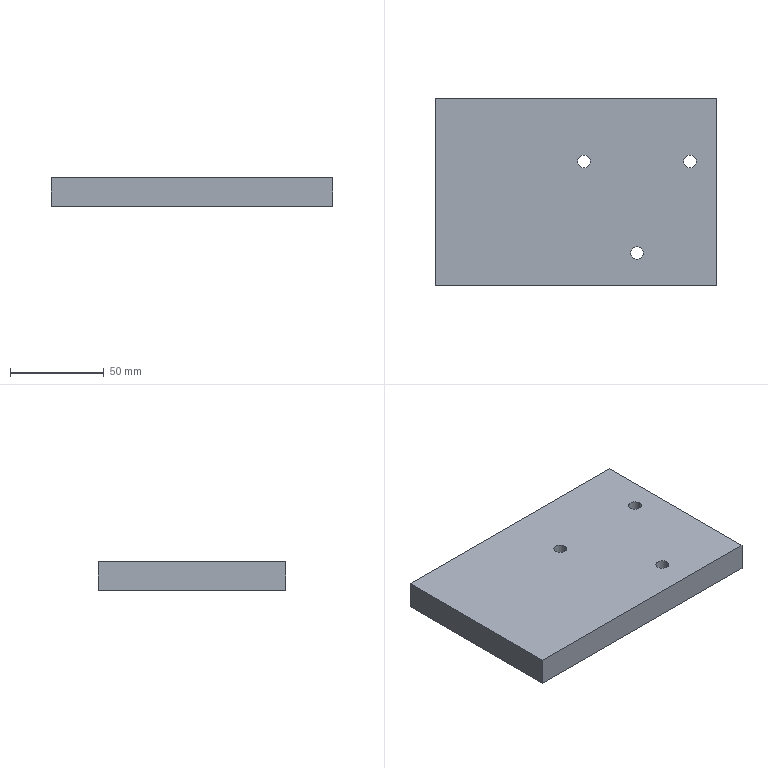Part | SolidWorks | features Extrusion 1, HoleWzd 1 | 1 solid | 12 faces | box 150 x 100 x 15 mm | volume 223366 mm3 | cylinder 6 | plane 6 | commonest cylinder face diameters 6.8 x6
STEP:
#1=CARTESIAN_POINT('',(0.9542,16.25,0.));
#2=VERTEX_POINT('',#1);
#3=CARTESIAN_POINT('',(7.754,16.25,0.));
#4=VERTEX_POINT('',#3);
#5=CARTESIAN_POINT('',(4.354,16.25,0.));
#6=DIRECTION('',(0.,0.,1.));
#7=DIRECTION('',(1.,0.,0.));
#8=AXIS2_PLACEMENT_3D('',#5,#6,#7);
#9=CIRCLE('',#8,3.4);
#10=EDGE_CURVE('',#2,#4,#9,.T.);
#11=ORIENTED_EDGE('',*,*,#10,.F.);
#12=CARTESIAN_POINT('',(0.9542,16.25,15.));
#13=VERTEX_POINT('',#12);
#14=CARTESIAN_POINT('',(0.9542,16.25,15.));
#15=DIRECTION('',(0.,0.,1.));
#16=VECTOR('',#15,1000.);
#17=LINE('',#14,#16);
#18=EDGE_CURVE('',#2,#13,#17,.T.);
#19=ORIENTED_EDGE('',*,*,#18,.T.);
#20=CARTESIAN_POINT('',(7.754,16.25,15.));
#21=VERTEX_POINT('',#20);
#22=CARTESIAN_POINT('',(4.354,16.25,15.));
#23=DIRECTION('',(0.,0.,1.));
#24=DIRECTION('',(1.,0.,0.));
#25=AXIS2_PLACEMENT_3D('',#22,#23,#24);
#26=CIRCLE('',#25,3.4);
#27=EDGE_CURVE('',#13,#21,#26,.T.);
#28=ORIENTED_EDGE('',*,*,#27,.T.);
#29=CARTESIAN_POINT('',(7.754,16.25,15.));
#30=DIRECTION('',(0.,0.,1.));
#31=VECTOR('',#30,1000.);
#32=LINE('',#29,#31);
#33=EDGE_CURVE('',#4,#21,#32,.T.);
#34=ORIENTED_EDGE('',*,*,#33,.F.);
#35=EDGE_LOOP('',(#11,#19,#28,#34));
#36=FACE_OUTER_BOUND('',#35,.T.);
#37=CARTESIAN_POINT('',(4.354,16.25,15.));
#38=DIRECTION('',(0.,0.,1.));
#39=DIRECTION('',(1.,0.,0.));
#40=AXIS2_PLACEMENT_3D('',#37,#38,#39);
#41=CYLINDRICAL_SURFACE('',#40,3.4);
#42=ADVANCED_FACE('',(#36),#41,.F.);
#43=CARTESIAN_POINT('',(57.246,16.25,0.));
#44=VERTEX_POINT('',#43);
#45=CARTESIAN_POINT('',(64.046,16.25,0.));
#46=VERTEX_POINT('',#45);
#47=CARTESIAN_POINT('',(60.646,16.25,0.));
#48=DIRECTION('',(0.,0.,1.));
#49=DIRECTION('',(1.,0.,0.));
#50=AXIS2_PLACEMENT_3D('',#47,#48,#49);
#51=CIRCLE('',#50,3.4);
#52=EDGE_CURVE('',#44,#46,#51,.T.);
#53=ORIENTED_EDGE('',*,*,#52,.F.);
#54=CARTESIAN_POINT('',(57.246,16.25,15.));
#55=VERTEX_POINT('',#54);
#56=CARTESIAN_POINT('',(57.246,16.25,15.));
#57=DIRECTION('',(0.,0.,1.));
#58=VECTOR('',#57,1000.);
#59=LINE('',#56,#58);
#60=EDGE_CURVE('',#44,#55,#59,.T.);
#61=ORIENTED_EDGE('',*,*,#60,.T.);
#62=CARTESIAN_POINT('',(64.046,16.25,15.));
#63=VERTEX_POINT('',#62);
#64=CARTESIAN_POINT('',(60.646,16.25,15.));
#65=DIRECTION('',(0.,0.,1.));
#66=DIRECTION('',(1.,0.,0.));
#67=AXIS2_PLACEMENT_3D('',#64,#65,#66);
#68=CIRCLE('',#67,3.4);
#69=EDGE_CURVE('',#55,#63,#68,.T.);
#70=ORIENTED_EDGE('',*,*,#69,.T.);
#71=CARTESIAN_POINT('',(64.046,16.25,15.));
#72=DIRECTION('',(0.,0.,1.));
#73=VECTOR('',#72,1000.);
#74=LINE('',#71,#73);
#75=EDGE_CURVE('',#46,#63,#74,.T.);
#76=ORIENTED_EDGE('',*,*,#75,.F.);
#77=EDGE_LOOP('',(#53,#61,#70,#76));
#78=FACE_OUTER_BOUND('',#77,.T.);
#79=CARTESIAN_POINT('',(60.646,16.25,15.));
#80=DIRECTION('',(0.,0.,1.));
#81=DIRECTION('',(1.,0.,0.));
#82=AXIS2_PLACEMENT_3D('',#79,#80,#81);
#83=CYLINDRICAL_SURFACE('',#82,3.4);
#84=ADVANCED_FACE('',(#78),#83,.F.);
#85=CARTESIAN_POINT('',(29.1,-32.5,0.));
#86=VERTEX_POINT('',#85);
#87=CARTESIAN_POINT('',(35.9,-32.5,0.));
#88=VERTEX_POINT('',#87);
#89=CARTESIAN_POINT('',(32.5,-32.5,0.));
#90=DIRECTION('',(0.,0.,1.));
#91=DIRECTION('',(1.,0.,0.));
#92=AXIS2_PLACEMENT_3D('',#89,#90,#91);
#93=CIRCLE('',#92,3.4);
#94=EDGE_CURVE('',#86,#88,#93,.T.);
#95=ORIENTED_EDGE('',*,*,#94,.F.);
#96=CARTESIAN_POINT('',(29.1,-32.5,15.));
#97=VERTEX_POINT('',#96);
#98=CARTESIAN_POINT('',(29.1,-32.5,15.));
#99=DIRECTION('',(0.,0.,1.));
#100=VECTOR('',#99,1000.);
#101=LINE('',#98,#100);
#102=EDGE_CURVE('',#86,#97,#101,.T.);
#103=ORIENTED_EDGE('',*,*,#102,.T.);
#104=CARTESIAN_POINT('',(35.9,-32.5,15.));
#105=VERTEX_POINT('',#104);
#106=CARTESIAN_POINT('',(32.5,-32.5,15.));
#107=DIRECTION('',(0.,0.,1.));
#108=DIRECTION('',(1.,0.,0.));
#109=AXIS2_PLACEMENT_3D('',#106,#107,#108);
#110=CIRCLE('',#109,3.4);
#111=EDGE_CURVE('',#97,#105,#110,.T.);
#112=ORIENTED_EDGE('',*,*,#111,.T.);
#113=CARTESIAN_POINT('',(35.9,-32.5,15.));
#114=DIRECTION('',(0.,0.,1.));
#115=VECTOR('',#114,1000.);
#116=LINE('',#113,#115);
#117=EDGE_CURVE('',#88,#105,#116,.T.);
#118=ORIENTED_EDGE('',*,*,#117,.F.);
#119=EDGE_LOOP('',(#95,#103,#112,#118));
#120=FACE_OUTER_BOUND('',#119,.T.);
#121=CARTESIAN_POINT('',(32.5,-32.5,15.));
#122=DIRECTION('',(0.,0.,1.));
#123=DIRECTION('',(1.,0.,0.));
#124=AXIS2_PLACEMENT_3D('',#121,#122,#123);
#125=CYLINDRICAL_SURFACE('',#124,3.4);
#126=ADVANCED_FACE('',(#120),#125,.F.);
#127=CARTESIAN_POINT('',(75.,-50.,0.));
#128=VERTEX_POINT('',#127);
#129=CARTESIAN_POINT('',(75.,50.,0.));
#130=VERTEX_POINT('',#129);
#131=CARTESIAN_POINT('',(75.,50.,0.));
#132=DIRECTION('',(0.,1.,0.));
#133=VECTOR('',#132,1000.);
#134=LINE('',#131,#133);
#135=EDGE_CURVE('',#128,#130,#134,.T.);
#136=ORIENTED_EDGE('',*,*,#135,.T.);
#137=CARTESIAN_POINT('',(75.,50.,15.));
#138=VERTEX_POINT('',#137);
#139=CARTESIAN_POINT('',(75.,50.,15.));
#140=DIRECTION('',(0.,0.,-1.));
#141=VECTOR('',#140,1000.);
#142=LINE('',#139,#141);
#143=EDGE_CURVE('',#138,#130,#142,.T.);
#144=ORIENTED_EDGE('',*,*,#143,.F.);
#145=CARTESIAN_POINT('',(75.,-50.,15.));
#146=VERTEX_POINT('',#145);
#147=CARTESIAN_POINT('',(75.,50.,15.));
#148=DIRECTION('',(0.,1.,0.));
#149=VECTOR('',#148,1000.);
#150=LINE('',#147,#149);
#151=EDGE_CURVE('',#146,#138,#150,.T.);
#152=ORIENTED_EDGE('',*,*,#151,.F.);
#153=CARTESIAN_POINT('',(75.,-50.,15.));
#154=DIRECTION('',(0.,0.,-1.));
#155=VECTOR('',#154,1000.);
#156=LINE('',#153,#155);
#157=EDGE_CURVE('',#146,#128,#156,.T.);
#158=ORIENTED_EDGE('',*,*,#157,.T.);
#159=EDGE_LOOP('',(#136,#144,#152,#158));
#160=FACE_OUTER_BOUND('',#159,.T.);
#161=CARTESIAN_POINT('',(75.,50.,15.));
#162=DIRECTION('',(-1.,0.,0.));
#163=DIRECTION('',(0.,-1.,0.));
#164=AXIS2_PLACEMENT_3D('',#161,#162,#163);
#165=PLANE('',#164);
#166=ADVANCED_FACE('',(#160),#165,.F.);
#167=CARTESIAN_POINT('',(-75.,50.,0.));
#168=VERTEX_POINT('',#167);
#169=CARTESIAN_POINT('',(-75.,50.,0.));
#170=DIRECTION('',(-1.,0.,0.));
#171=VECTOR('',#170,1000.);
#172=LINE('',#169,#171);
#173=EDGE_CURVE('',#130,#168,#172,.T.);
#174=ORIENTED_EDGE('',*,*,#173,.T.);
#175=CARTESIAN_POINT('',(-75.,50.,15.));
#176=VERTEX_POINT('',#175);
#177=CARTESIAN_POINT('',(-75.,50.,15.));
#178=DIRECTION('',(0.,0.,-1.));
#179=VECTOR('',#178,1000.);
#180=LINE('',#177,#179);
#181=EDGE_CURVE('',#176,#168,#180,.T.);
#182=ORIENTED_EDGE('',*,*,#181,.F.);
#183=CARTESIAN_POINT('',(-75.,50.,15.));
#184=DIRECTION('',(-1.,0.,0.));
#185=VECTOR('',#184,1000.);
#186=LINE('',#183,#185);
#187=EDGE_CURVE('',#138,#176,#186,.T.);
#188=ORIENTED_EDGE('',*,*,#187,.F.);
#189=ORIENTED_EDGE('',*,*,#143,.T.);
#190=EDGE_LOOP('',(#174,#182,#188,#189));
#191=FACE_OUTER_BOUND('',#190,.T.);
#192=CARTESIAN_POINT('',(-75.,50.,15.));
#193=DIRECTION('',(0.,-1.,0.));
#194=DIRECTION('',(0.,0.,-1.));
#195=AXIS2_PLACEMENT_3D('',#192,#193,#194);
#196=PLANE('',#195);
#197=ADVANCED_FACE('',(#191),#196,.F.);
#198=CARTESIAN_POINT('',(-75.,-50.,0.));
#199=VERTEX_POINT('',#198);
#200=CARTESIAN_POINT('',(-75.,50.,0.));
#201=DIRECTION('',(0.,-1.,0.));
#202=VECTOR('',#201,1000.);
#203=LINE('',#200,#202);
#204=EDGE_CURVE('',#168,#199,#203,.T.);
#205=ORIENTED_EDGE('',*,*,#204,.T.);
#206=CARTESIAN_POINT('',(-75.,-50.,15.));
#207=VERTEX_POINT('',#206);
#208=CARTESIAN_POINT('',(-75.,-50.,15.));
#209=DIRECTION('',(0.,0.,-1.));
#210=VECTOR('',#209,1000.);
#211=LINE('',#208,#210);
#212=EDGE_CURVE('',#207,#199,#211,.T.);
#213=ORIENTED_EDGE('',*,*,#212,.F.);
#214=CARTESIAN_POINT('',(-75.,50.,15.));
#215=DIRECTION('',(0.,-1.,0.));
#216=VECTOR('',#215,1000.);
#217=LINE('',#214,#216);
#218=EDGE_CURVE('',#176,#207,#217,.T.);
#219=ORIENTED_EDGE('',*,*,#218,.F.);
#220=ORIENTED_EDGE('',*,*,#181,.T.);
#221=EDGE_LOOP('',(#205,#213,#219,#220));
#222=FACE_OUTER_BOUND('',#221,.T.);
#223=CARTESIAN_POINT('',(-75.,50.,15.));
#224=DIRECTION('',(1.,0.,0.));
#225=DIRECTION('',(0.,0.,-1.));
#226=AXIS2_PLACEMENT_3D('',#223,#224,#225);
#227=PLANE('',#226);
#228=ADVANCED_FACE('',(#222),#227,.F.);
#229=CARTESIAN_POINT('',(-75.,-50.,0.));
#230=DIRECTION('',(1.,0.,0.));
#231=VECTOR('',#230,1000.);
#232=LINE('',#229,#231);
#233=EDGE_CURVE('',#199,#128,#232,.T.);
#234=ORIENTED_EDGE('',*,*,#233,.T.);
#235=ORIENTED_EDGE('',*,*,#157,.F.);
#236=CARTESIAN_POINT('',(-75.,-50.,15.));
#237=DIRECTION('',(1.,0.,0.));
#238=VECTOR('',#237,1000.);
#239=LINE('',#236,#238);
#240=EDGE_CURVE('',#207,#146,#239,.T.);
#241=ORIENTED_EDGE('',*,*,#240,.F.);
#242=ORIENTED_EDGE('',*,*,#212,.T.);
#243=EDGE_LOOP('',(#234,#235,#241,#242));
#244=FACE_OUTER_BOUND('',#243,.T.);
#245=CARTESIAN_POINT('',(-75.,-50.,15.));
#246=DIRECTION('',(0.,1.,0.));
#247=DIRECTION('',(0.,0.,1.));
#248=AXIS2_PLACEMENT_3D('',#245,#246,#247);
#249=PLANE('',#248);
#250=ADVANCED_FACE('',(#244),#249,.F.);
#251=CARTESIAN_POINT('',(4.354,16.25,15.));
#252=DIRECTION('',(0.,0.,1.));
#253=DIRECTION('',(1.,0.,0.));
#254=AXIS2_PLACEMENT_3D('',#251,#252,#253);
#255=CIRCLE('',#254,3.4);
#256=EDGE_CURVE('',#21,#13,#255,.T.);
#257=ORIENTED_EDGE('',*,*,#256,.F.);
#258=ORIENTED_EDGE('',*,*,#27,.F.);
#259=EDGE_LOOP('',(#257,#258));
#260=FACE_BOUND('',#259,.T.);
#261=CARTESIAN_POINT('',(60.646,16.25,15.));
#262=DIRECTION('',(0.,0.,1.));
#263=DIRECTION('',(1.,0.,0.));
#264=AXIS2_PLACEMENT_3D('',#261,#262,#263);
#265=CIRCLE('',#264,3.4);
#266=EDGE_CURVE('',#63,#55,#265,.T.);
#267=ORIENTED_EDGE('',*,*,#266,.F.);
#268=ORIENTED_EDGE('',*,*,#69,.F.);
#269=EDGE_LOOP('',(#267,#268));
#270=FACE_BOUND('',#269,.T.);
#271=CARTESIAN_POINT('',(32.5,-32.5,15.));
#272=DIRECTION('',(0.,0.,1.));
#273=DIRECTION('',(1.,0.,0.));
#274=AXIS2_PLACEMENT_3D('',#271,#272,#273);
#275=CIRCLE('',#274,3.4);
#276=EDGE_CURVE('',#105,#97,#275,.T.);
#277=ORIENTED_EDGE('',*,*,#276,.F.);
#278=ORIENTED_EDGE('',*,*,#111,.F.);
#279=EDGE_LOOP('',(#277,#278));
#280=FACE_BOUND('',#279,.T.);
#281=ORIENTED_EDGE('',*,*,#151,.T.);
#282=ORIENTED_EDGE('',*,*,#187,.T.);
#283=ORIENTED_EDGE('',*,*,#218,.T.);
#284=ORIENTED_EDGE('',*,*,#240,.T.);
#285=EDGE_LOOP('',(#281,#282,#283,#284));
#286=FACE_OUTER_BOUND('',#285,.T.);
#287=CARTESIAN_POINT('',(0.,0.,15.));
#288=DIRECTION('',(0.,0.,1.));
#289=DIRECTION('',(1.,0.,0.));
#290=AXIS2_PLACEMENT_3D('',#287,#288,#289);
#291=PLANE('',#290);
#292=ADVANCED_FACE('',(#260,#270,#280,#286),#291,.T.);
#293=CARTESIAN_POINT('',(4.354,16.25,0.));
#294=DIRECTION('',(0.,0.,1.));
#295=DIRECTION('',(1.,0.,0.));
#296=AXIS2_PLACEMENT_3D('',#293,#294,#295);
#297=CIRCLE('',#296,3.4);
#298=EDGE_CURVE('',#4,#2,#297,.T.);
#299=ORIENTED_EDGE('',*,*,#298,.T.);
#300=ORIENTED_EDGE('',*,*,#10,.T.);
#301=EDGE_LOOP('',(#299,#300));
#302=FACE_BOUND('',#301,.T.);
#303=CARTESIAN_POINT('',(60.646,16.25,0.));
#304=DIRECTION('',(0.,0.,1.));
#305=DIRECTION('',(1.,0.,0.));
#306=AXIS2_PLACEMENT_3D('',#303,#304,#305);
#307=CIRCLE('',#306,3.4);
#308=EDGE_CURVE('',#46,#44,#307,.T.);
#309=ORIENTED_EDGE('',*,*,#308,.T.);
#310=ORIENTED_EDGE('',*,*,#52,.T.);
#311=EDGE_LOOP('',(#309,#310));
#312=FACE_BOUND('',#311,.T.);
#313=CARTESIAN_POINT('',(32.5,-32.5,0.));
#314=DIRECTION('',(0.,0.,1.));
#315=DIRECTION('',(1.,0.,0.));
#316=AXIS2_PLACEMENT_3D('',#313,#314,#315);
#317=CIRCLE('',#316,3.4);
#318=EDGE_CURVE('',#88,#86,#317,.T.);
#319=ORIENTED_EDGE('',*,*,#318,.T.);
#320=ORIENTED_EDGE('',*,*,#94,.T.);
#321=EDGE_LOOP('',(#319,#320));
#322=FACE_BOUND('',#321,.T.);
#323=ORIENTED_EDGE('',*,*,#135,.F.);
#324=ORIENTED_EDGE('',*,*,#233,.F.);
#325=ORIENTED_EDGE('',*,*,#204,.F.);
#326=ORIENTED_EDGE('',*,*,#173,.F.);
#327=EDGE_LOOP('',(#323,#324,#325,#326));
#328=FACE_OUTER_BOUND('',#327,.T.);
#329=CARTESIAN_POINT('',(0.,0.,0.));
#330=DIRECTION('',(0.,0.,1.));
#331=DIRECTION('',(1.,0.,0.));
#332=AXIS2_PLACEMENT_3D('',#329,#330,#331);
#333=PLANE('',#332);
#334=ADVANCED_FACE('',(#302,#312,#322,#328),#333,.F.);
#335=ORIENTED_EDGE('',*,*,#102,.F.);
#336=ORIENTED_EDGE('',*,*,#318,.F.);
#337=ORIENTED_EDGE('',*,*,#117,.T.);
#338=ORIENTED_EDGE('',*,*,#276,.T.);
#339=EDGE_LOOP('',(#335,#336,#337,#338));
#340=FACE_OUTER_BOUND('',#339,.T.);
#341=CARTESIAN_POINT('',(32.5,-32.5,15.));
#342=DIRECTION('',(0.,0.,1.));
#343=DIRECTION('',(1.,0.,0.));
#344=AXIS2_PLACEMENT_3D('',#341,#342,#343);
#345=CYLINDRICAL_SURFACE('',#344,3.4);
#346=ADVANCED_FACE('',(#340),#345,.F.);
#347=ORIENTED_EDGE('',*,*,#60,.F.);
#348=ORIENTED_EDGE('',*,*,#308,.F.);
#349=ORIENTED_EDGE('',*,*,#75,.T.);
#350=ORIENTED_EDGE('',*,*,#266,.T.);
#351=EDGE_LOOP('',(#347,#348,#349,#350));
#352=FACE_OUTER_BOUND('',#351,.T.);
#353=CARTESIAN_POINT('',(60.646,16.25,15.));
#354=DIRECTION('',(0.,0.,1.));
#355=DIRECTION('',(1.,0.,0.));
#356=AXIS2_PLACEMENT_3D('',#353,#354,#355);
#357=CYLINDRICAL_SURFACE('',#356,3.4);
#358=ADVANCED_FACE('',(#352),#357,.F.);
#359=ORIENTED_EDGE('',*,*,#18,.F.);
#360=ORIENTED_EDGE('',*,*,#298,.F.);
#361=ORIENTED_EDGE('',*,*,#33,.T.);
#362=ORIENTED_EDGE('',*,*,#256,.T.);
#363=EDGE_LOOP('',(#359,#360,#361,#362));
#364=FACE_OUTER_BOUND('',#363,.T.);
#365=CARTESIAN_POINT('',(4.354,16.25,15.));
#366=DIRECTION('',(0.,0.,1.));
#367=DIRECTION('',(1.,0.,0.));
#368=AXIS2_PLACEMENT_3D('',#365,#366,#367);
#369=CYLINDRICAL_SURFACE('',#368,3.4);
#370=ADVANCED_FACE('',(#364),#369,.F.);
#371=CLOSED_SHELL('',(#42,#84,#126,#166,#197,#228,#250,#292,#334,#346,#358,#370));
#372=MANIFOLD_SOLID_BREP('',#371);
#373=CARTESIAN_POINT('',(0.,0.,0.));
#374=DIRECTION('',(0.,0.,1.));
#375=DIRECTION('',(1.,0.,0.));
#376=AXIS2_PLACEMENT_3D('',#373,#374,#375);
#377=(LENGTH_UNIT()NAMED_UNIT(*)SI_UNIT(.MILLI.,.METRE.));
#378=UNCERTAINTY_MEASURE_WITH_UNIT(LENGTH_MEASURE(0.00001),#377,'','');
#379=(NAMED_UNIT(*)PLANE_ANGLE_UNIT()SI_UNIT($,.RADIAN.));
#380=(NAMED_UNIT(*)SI_UNIT($,.STERADIAN.)SOLID_ANGLE_UNIT());
#381=(GEOMETRIC_REPRESENTATION_CONTEXT(3)GLOBAL_UNCERTAINTY_ASSIGNED_CONTEXT((#378))GLOBAL_UNIT_ASSIGNED_CONTEXT((#377,#379,#380))REPRESENTATION_CONTEXT('',''));
#382=ADVANCED_BREP_SHAPE_REPRESENTATION('',(#372,#376),#381);